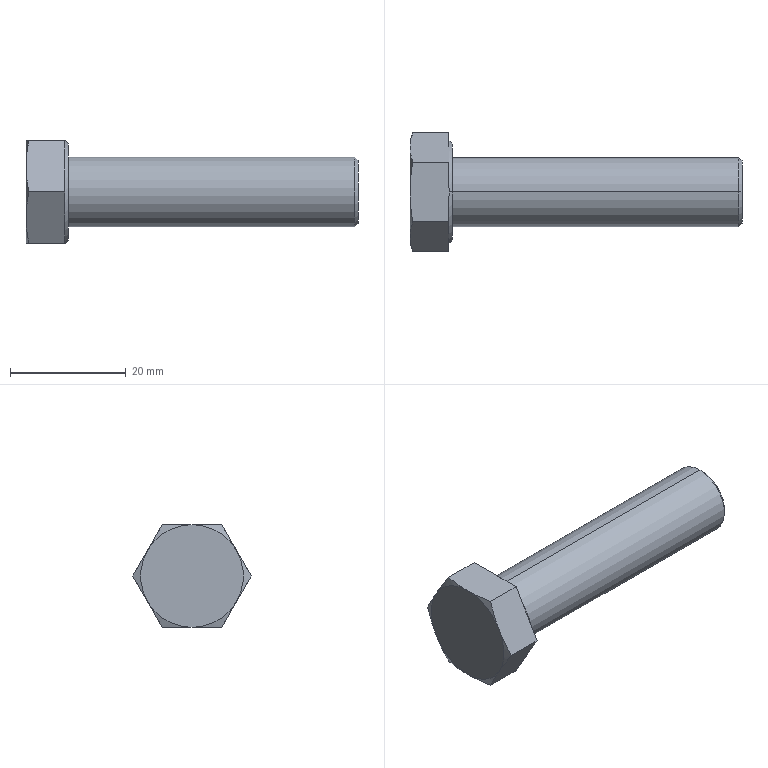Part | SolidWorks | features RevCut 3, Boss 1, Chamfer 1, Extrusion 1, Fillet 1, LPattern 1 | 1 solid | 27 faces | box 57.32 x 20.473 x 17.73 mm | volume 7614 mm3 | plane 15 | cone 10 | cylinder 2 | commonest cylinder face diameters 12 x2
STEP:
#1=CARTESIAN_POINT('',(57.32,0.,-5.4));
#2=VERTEX_POINT('',#1);
#3=CARTESIAN_POINT('',(57.32,0.,5.4));
#4=VERTEX_POINT('',#3);
#5=CARTESIAN_POINT('',(57.32,0.,0.));
#6=DIRECTION('',(1.,0.,0.));
#7=DIRECTION('',(0.,0.,-1.));
#8=AXIS2_PLACEMENT_3D('',#5,#6,#7);
#9=CIRCLE('',#8,5.4);
#10=EDGE_CURVE('',#2,#4,#9,.T.);
#11=ORIENTED_EDGE('',*,*,#10,.F.);
#12=CARTESIAN_POINT('',(56.72,0.,-6.));
#13=VERTEX_POINT('',#12);
#14=CARTESIAN_POINT('',(57.32,0.,-5.4));
#15=DIRECTION('',(-0.7071,0.,-0.7071));
#16=VECTOR('',#15,1000.);
#17=LINE('',#14,#16);
#18=EDGE_CURVE('',#2,#13,#17,.T.);
#19=ORIENTED_EDGE('',*,*,#18,.T.);
#20=CARTESIAN_POINT('',(56.72,0.,6.));
#21=VERTEX_POINT('',#20);
#22=CARTESIAN_POINT('',(56.72,0.,0.));
#23=DIRECTION('',(-1.,0.,0.));
#24=DIRECTION('',(0.,0.,-1.));
#25=AXIS2_PLACEMENT_3D('',#22,#23,#24);
#26=CIRCLE('',#25,6.);
#27=EDGE_CURVE('',#21,#13,#26,.T.);
#28=ORIENTED_EDGE('',*,*,#27,.F.);
#29=CARTESIAN_POINT('',(57.32,0.,5.4));
#30=DIRECTION('',(-0.7071,0.,0.7071));
#31=VECTOR('',#30,1000.);
#32=LINE('',#29,#31);
#33=EDGE_CURVE('',#4,#21,#32,.T.);
#34=ORIENTED_EDGE('',*,*,#33,.F.);
#35=EDGE_LOOP('',(#11,#19,#28,#34));
#36=FACE_OUTER_BOUND('',#35,.T.);
#37=CARTESIAN_POINT('',(57.32,0.,0.));
#38=DIRECTION('',(-1.,0.,0.));
#39=DIRECTION('',(0.,0.,1.));
#40=AXIS2_PLACEMENT_3D('',#37,#38,#39);
#41=CONICAL_SURFACE('',#40,5.4,0.7854);
#42=ADVANCED_FACE('',(#36),#41,.T.);
#43=ORIENTED_EDGE('',*,*,#27,.T.);
#44=CARTESIAN_POINT('',(7.32,0.,-6.));
#45=VERTEX_POINT('',#44);
#46=CARTESIAN_POINT('',(57.32,0.,-6.));
#47=DIRECTION('',(-1.,0.,0.));
#48=VECTOR('',#47,1000.);
#49=LINE('',#46,#48);
#50=EDGE_CURVE('',#13,#45,#49,.T.);
#51=ORIENTED_EDGE('',*,*,#50,.T.);
#52=CARTESIAN_POINT('',(7.32,0.,6.));
#53=VERTEX_POINT('',#52);
#54=CARTESIAN_POINT('',(7.32,0.,0.));
#55=DIRECTION('',(1.,0.,0.));
#56=DIRECTION('',(0.,0.,-1.));
#57=AXIS2_PLACEMENT_3D('',#54,#55,#56);
#58=CIRCLE('',#57,6.);
#59=EDGE_CURVE('',#45,#53,#58,.T.);
#60=ORIENTED_EDGE('',*,*,#59,.T.);
#61=CARTESIAN_POINT('',(57.32,0.,6.));
#62=DIRECTION('',(-1.,0.,0.));
#63=VECTOR('',#62,1000.);
#64=LINE('',#61,#63);
#65=EDGE_CURVE('',#21,#53,#64,.T.);
#66=ORIENTED_EDGE('',*,*,#65,.F.);
#67=EDGE_LOOP('',(#43,#51,#60,#66));
#68=FACE_OUTER_BOUND('',#67,.T.);
#69=CARTESIAN_POINT('',(57.32,0.,0.));
#70=DIRECTION('',(-1.,0.,0.));
#71=DIRECTION('',(0.,0.,1.));
#72=AXIS2_PLACEMENT_3D('',#69,#70,#71);
#73=CYLINDRICAL_SURFACE('',#72,6.);
#74=ADVANCED_FACE('',(#68),#73,.T.);
#75=CARTESIAN_POINT('',(7.32,0.,8.315));
#76=VERTEX_POINT('',#75);
#77=CARTESIAN_POINT('',(7.32,0.,-8.315));
#78=VERTEX_POINT('',#77);
#79=CARTESIAN_POINT('',(7.32,0.,0.));
#80=DIRECTION('',(-1.,0.,0.));
#81=DIRECTION('',(0.,0.,1.));
#82=AXIS2_PLACEMENT_3D('',#79,#80,#81);
#83=CIRCLE('',#82,8.315);
#84=EDGE_CURVE('',#76,#78,#83,.T.);
#85=ORIENTED_EDGE('',*,*,#84,.T.);
#86=CARTESIAN_POINT('',(6.77,0.,-8.865));
#87=VERTEX_POINT('',#86);
#88=CARTESIAN_POINT('',(6.72,0.,-8.915));
#89=DIRECTION('',(-0.7071,0.,-0.7071));
#90=VECTOR('',#89,1000.);
#91=LINE('',#88,#90);
#92=EDGE_CURVE('',#78,#87,#91,.T.);
#93=ORIENTED_EDGE('',*,*,#92,.T.);
#94=CARTESIAN_POINT('',(6.72,0.9429,-8.865));
#95=VERTEX_POINT('',#94);
#96=CARTESIAN_POINT('',(6.77,0.,-8.865));
#97=CARTESIAN_POINT('',(6.77,0.3145,-8.865));
#98=CARTESIAN_POINT('',(6.753,0.6288,-8.865));
#99=CARTESIAN_POINT('',(6.72,0.9429,-8.865));
#100=B_SPLINE_CURVE_WITH_KNOTS('',3,(#96,#97,#98,#99),.UNSPECIFIED.,.F.,.F.,(4,4),(0.004972,0.005912),.UNSPECIFIED.);
#101=EDGE_CURVE('',#87,#95,#100,.T.);
#102=ORIENTED_EDGE('',*,*,#101,.T.);
#103=CARTESIAN_POINT('',(6.72,7.206,-5.249));
#104=VERTEX_POINT('',#103);
#105=CARTESIAN_POINT('',(6.72,0.,0.));
#106=DIRECTION('',(-1.,0.,0.));
#107=DIRECTION('',(0.,0.,1.));
#108=AXIS2_PLACEMENT_3D('',#105,#106,#107);
#109=CIRCLE('',#108,8.915);
#110=EDGE_CURVE('',#104,#95,#109,.T.);
#111=ORIENTED_EDGE('',*,*,#110,.F.);
#112=CARTESIAN_POINT('',(6.72,8.149,-3.616));
#113=VERTEX_POINT('',#112);
#114=CARTESIAN_POINT('',(6.72,7.206,-5.249));
#115=CARTESIAN_POINT('',(6.786,7.52,-4.705));
#116=CARTESIAN_POINT('',(6.786,7.834,-4.16));
#117=CARTESIAN_POINT('',(6.72,8.149,-3.616));
#118=B_SPLINE_CURVE_WITH_KNOTS('',3,(#114,#115,#116,#117),.UNSPECIFIED.,.F.,.F.,(4,4),(0.000001889,0.001888),.UNSPECIFIED.);
#119=EDGE_CURVE('',#104,#113,#118,.T.);
#120=ORIENTED_EDGE('',*,*,#119,.T.);
#121=CARTESIAN_POINT('',(6.72,8.149,3.616));
#122=VERTEX_POINT('',#121);
#123=CARTESIAN_POINT('',(6.72,0.,0.));
#124=DIRECTION('',(-1.,0.,0.));
#125=DIRECTION('',(0.,0.,1.));
#126=AXIS2_PLACEMENT_3D('',#123,#124,#125);
#127=CIRCLE('',#126,8.915);
#128=EDGE_CURVE('',#122,#113,#127,.T.);
#129=ORIENTED_EDGE('',*,*,#128,.F.);
#130=CARTESIAN_POINT('',(6.72,7.206,5.249));
#131=VERTEX_POINT('',#130);
#132=CARTESIAN_POINT('',(6.72,8.149,3.616));
#133=CARTESIAN_POINT('',(6.786,7.834,4.16));
#134=CARTESIAN_POINT('',(6.786,7.52,4.705));
#135=CARTESIAN_POINT('',(6.72,7.206,5.249));
#136=B_SPLINE_CURVE_WITH_KNOTS('',3,(#132,#133,#134,#135),.UNSPECIFIED.,.F.,.F.,(4,4),(0.000001889,0.001888),.UNSPECIFIED.);
#137=EDGE_CURVE('',#122,#131,#136,.T.);
#138=ORIENTED_EDGE('',*,*,#137,.T.);
#139=CARTESIAN_POINT('',(6.72,0.9429,8.865));
#140=VERTEX_POINT('',#139);
#141=CARTESIAN_POINT('',(6.72,0.,0.));
#142=DIRECTION('',(-1.,0.,0.));
#143=DIRECTION('',(0.,0.,1.));
#144=AXIS2_PLACEMENT_3D('',#141,#142,#143);
#145=CIRCLE('',#144,8.915);
#146=EDGE_CURVE('',#140,#131,#145,.T.);
#147=ORIENTED_EDGE('',*,*,#146,.F.);
#148=CARTESIAN_POINT('',(6.77,0.,8.865));
#149=VERTEX_POINT('',#148);
#150=CARTESIAN_POINT('',(6.72,0.9429,8.865));
#151=CARTESIAN_POINT('',(6.753,0.6288,8.865));
#152=CARTESIAN_POINT('',(6.77,0.3145,8.865));
#153=CARTESIAN_POINT('',(6.77,0.,8.865));
#154=B_SPLINE_CURVE_WITH_KNOTS('',3,(#150,#151,#152,#153),.UNSPECIFIED.,.F.,.F.,(4,4),(0.004457,0.005396),.UNSPECIFIED.);
#155=EDGE_CURVE('',#140,#149,#154,.T.);
#156=ORIENTED_EDGE('',*,*,#155,.T.);
#157=CARTESIAN_POINT('',(6.72,0.,8.915));
#158=DIRECTION('',(-0.7071,0.,0.7071));
#159=VECTOR('',#158,1000.);
#160=LINE('',#157,#159);
#161=EDGE_CURVE('',#76,#149,#160,.T.);
#162=ORIENTED_EDGE('',*,*,#161,.F.);
#163=EDGE_LOOP('',(#85,#93,#102,#111,#120,#129,#138,#147,#156,#162));
#164=FACE_OUTER_BOUND('',#163,.T.);
#165=CARTESIAN_POINT('',(6.72,0.,0.));
#166=DIRECTION('',(-1.,0.,0.));
#167=DIRECTION('',(0.,0.,1.));
#168=AXIS2_PLACEMENT_3D('',#165,#166,#167);
#169=CONICAL_SURFACE('',#168,8.915,0.7854);
#170=ADVANCED_FACE('',(#164),#169,.T.);
#171=ORIENTED_EDGE('',*,*,#84,.F.);
#172=CARTESIAN_POINT('',(7.32,0.,0.));
#173=DIRECTION('',(-1.,0.,0.));
#174=DIRECTION('',(0.,0.,1.));
#175=AXIS2_PLACEMENT_3D('',#172,#173,#174);
#176=CIRCLE('',#175,8.315);
#177=EDGE_CURVE('',#78,#76,#176,.T.);
#178=ORIENTED_EDGE('',*,*,#177,.F.);
#179=EDGE_LOOP('',(#171,#178));
#180=FACE_OUTER_BOUND('',#179,.T.);
#181=CARTESIAN_POINT('',(7.32,0.,0.));
#182=DIRECTION('',(1.,0.,0.));
#183=DIRECTION('',(0.,0.,-1.));
#184=AXIS2_PLACEMENT_3D('',#181,#182,#183);
#185=CIRCLE('',#184,6.);
#186=EDGE_CURVE('',#53,#45,#185,.T.);
#187=ORIENTED_EDGE('',*,*,#186,.F.);
#188=ORIENTED_EDGE('',*,*,#59,.F.);
#189=EDGE_LOOP('',(#187,#188));
#190=FACE_BOUND('',#189,.T.);
#191=CARTESIAN_POINT('',(7.32,-15.355,-8.865));
#192=DIRECTION('',(1.,0.,0.));
#193=DIRECTION('',(0.,0.,-1.));
#194=AXIS2_PLACEMENT_3D('',#191,#192,#193);
#195=PLANE('',#194);
#196=ADVANCED_FACE('',(#180,#190),#195,.T.);
#197=CARTESIAN_POINT('',(0.4992,-10.236,0.));
#198=VERTEX_POINT('',#197);
#199=CARTESIAN_POINT('',(0.,-7.677,4.433));
#200=VERTEX_POINT('',#199);
#201=CARTESIAN_POINT('',(0.4992,-10.236,0.));
#202=CARTESIAN_POINT('',(0.3439,-9.81,0.7388));
#203=CARTESIAN_POINT('',(0.2179,-9.383,1.478));
#204=CARTESIAN_POINT('',(0.04564,-8.53,2.955));
#205=CARTESIAN_POINT('',(0.,-8.104,3.694));
#206=CARTESIAN_POINT('',(0.,-7.677,4.433));
#207=B_SPLINE_CURVE_WITH_KNOTS('',3,(#201,#202,#203,#204,#205,#206),.UNSPECIFIED.,.F.,.F.,(4,2,4),(0.000000231,0.002559,0.005118),.UNSPECIFIED.);
#208=EDGE_CURVE('',#198,#200,#207,.T.);
#209=ORIENTED_EDGE('',*,*,#208,.F.);
#210=CARTESIAN_POINT('',(6.72,-10.236,0.));
#211=VERTEX_POINT('',#210);
#212=CARTESIAN_POINT('',(7.32,-10.236,0.));
#213=DIRECTION('',(-1.,0.,0.));
#214=VECTOR('',#213,1000.);
#215=LINE('',#212,#214);
#216=EDGE_CURVE('',#211,#198,#215,.T.);
#217=ORIENTED_EDGE('',*,*,#216,.F.);
#218=CARTESIAN_POINT('',(6.72,-8.149,3.616));
#219=VERTEX_POINT('',#218);
#220=CARTESIAN_POINT('',(6.72,-5.118,8.865));
#221=DIRECTION('',(0.,-0.5,-0.866));
#222=VECTOR('',#221,1000.);
#223=LINE('',#220,#222);
#224=EDGE_CURVE('',#219,#211,#223,.T.);
#225=ORIENTED_EDGE('',*,*,#224,.F.);
#226=CARTESIAN_POINT('',(6.72,-7.206,5.249));
#227=VERTEX_POINT('',#226);
#228=CARTESIAN_POINT('',(6.72,-7.206,5.249));
#229=CARTESIAN_POINT('',(6.786,-7.52,4.705));
#230=CARTESIAN_POINT('',(6.786,-7.834,4.16));
#231=CARTESIAN_POINT('',(6.72,-8.149,3.616));
#232=B_SPLINE_CURVE_WITH_KNOTS('',3,(#228,#229,#230,#231),.UNSPECIFIED.,.F.,.F.,(4,4),(0.000001889,0.001888),.UNSPECIFIED.);
#233=EDGE_CURVE('',#227,#219,#232,.T.);
#234=ORIENTED_EDGE('',*,*,#233,.F.);
#235=CARTESIAN_POINT('',(6.72,-5.118,8.865));
#236=VERTEX_POINT('',#235);
#237=CARTESIAN_POINT('',(6.72,-5.118,8.865));
#238=DIRECTION('',(0.,-0.5,-0.866));
#239=VECTOR('',#238,1000.);
#240=LINE('',#237,#239);
#241=EDGE_CURVE('',#236,#227,#240,.T.);
#242=ORIENTED_EDGE('',*,*,#241,.F.);
#243=CARTESIAN_POINT('',(0.4992,-5.118,8.865));
#244=VERTEX_POINT('',#243);
#245=CARTESIAN_POINT('',(7.32,-5.118,8.865));
#246=DIRECTION('',(-1.,0.,0.));
#247=VECTOR('',#246,1000.);
#248=LINE('',#245,#247);
#249=EDGE_CURVE('',#236,#244,#248,.T.);
#250=ORIENTED_EDGE('',*,*,#249,.T.);
#251=CARTESIAN_POINT('',(0.,-7.677,4.433));
#252=CARTESIAN_POINT('',(0.,-7.251,5.171));
#253=CARTESIAN_POINT('',(0.04564,-6.824,5.91));
#254=CARTESIAN_POINT('',(0.2179,-5.971,7.387));
#255=CARTESIAN_POINT('',(0.3439,-5.545,8.126));
#256=CARTESIAN_POINT('',(0.4992,-5.118,8.865));
#257=B_SPLINE_CURVE_WITH_KNOTS('',3,(#251,#252,#253,#254,#255,#256),.UNSPECIFIED.,.F.,.F.,(4,2,4),(0.005118,0.007678,0.01024),.UNSPECIFIED.);
#258=EDGE_CURVE('',#200,#244,#257,.T.);
#259=ORIENTED_EDGE('',*,*,#258,.F.);
#260=EDGE_LOOP('',(#209,#217,#225,#234,#242,#250,#259));
#261=FACE_OUTER_BOUND('',#260,.T.);
#262=CARTESIAN_POINT('',(7.32,-5.118,8.865));
#263=DIRECTION('',(0.,0.866,-0.5));
#264=DIRECTION('',(0.,0.5,0.866));
#265=AXIS2_PLACEMENT_3D('',#262,#263,#264);
#266=PLANE('',#265);
#267=ADVANCED_FACE('',(#261),#266,.F.);
#268=CARTESIAN_POINT('',(0.4992,-5.118,-8.865));
#269=VERTEX_POINT('',#268);
#270=CARTESIAN_POINT('',(0.,-7.677,-4.432));
#271=VERTEX_POINT('',#270);
#272=CARTESIAN_POINT('',(0.4992,-5.118,-8.865));
#273=CARTESIAN_POINT('',(0.3439,-5.545,-8.126));
#274=CARTESIAN_POINT('',(0.2179,-5.971,-7.387));
#275=CARTESIAN_POINT('',(0.04564,-6.824,-5.91));
#276=CARTESIAN_POINT('',(0.,-7.251,-5.171));
#277=CARTESIAN_POINT('',(0.,-7.677,-4.432));
#278=B_SPLINE_CURVE_WITH_KNOTS('',3,(#272,#273,#274,#275,#276,#277),.UNSPECIFIED.,.F.,.F.,(4,2,4),(0.000000231,0.002559,0.005118),.UNSPECIFIED.);
#279=EDGE_CURVE('',#269,#271,#278,.T.);
#280=ORIENTED_EDGE('',*,*,#279,.F.);
#281=CARTESIAN_POINT('',(6.72,-5.118,-8.865));
#282=VERTEX_POINT('',#281);
#283=CARTESIAN_POINT('',(7.32,-5.118,-8.865));
#284=DIRECTION('',(-1.,0.,0.));
#285=VECTOR('',#284,1000.);
#286=LINE('',#283,#285);
#287=EDGE_CURVE('',#282,#269,#286,.T.);
#288=ORIENTED_EDGE('',*,*,#287,.F.);
#289=CARTESIAN_POINT('',(6.72,-7.206,-5.249));
#290=VERTEX_POINT('',#289);
#291=CARTESIAN_POINT('',(6.72,-10.236,0.));
#292=DIRECTION('',(0.,0.5,-0.866));
#293=VECTOR('',#292,1000.);
#294=LINE('',#291,#293);
#295=EDGE_CURVE('',#290,#282,#294,.T.);
#296=ORIENTED_EDGE('',*,*,#295,.F.);
#297=CARTESIAN_POINT('',(6.72,-8.149,-3.616));
#298=VERTEX_POINT('',#297);
#299=CARTESIAN_POINT('',(6.72,-8.149,-3.616));
#300=CARTESIAN_POINT('',(6.786,-7.834,-4.16));
#301=CARTESIAN_POINT('',(6.786,-7.52,-4.705));
#302=CARTESIAN_POINT('',(6.72,-7.206,-5.249));
#303=B_SPLINE_CURVE_WITH_KNOTS('',3,(#299,#300,#301,#302),.UNSPECIFIED.,.F.,.F.,(4,4),(0.000001889,0.001888),.UNSPECIFIED.);
#304=EDGE_CURVE('',#298,#290,#303,.T.);
#305=ORIENTED_EDGE('',*,*,#304,.F.);
#306=CARTESIAN_POINT('',(6.72,-10.236,0.));
#307=DIRECTION('',(0.,0.5,-0.866));
#308=VECTOR('',#307,1000.);
#309=LINE('',#306,#308);
#310=EDGE_CURVE('',#211,#298,#309,.T.);
#311=ORIENTED_EDGE('',*,*,#310,.F.);
#312=ORIENTED_EDGE('',*,*,#216,.T.);
#313=CARTESIAN_POINT('',(0.,-7.677,-4.432));
#314=CARTESIAN_POINT('',(0.,-8.104,-3.694));
#315=CARTESIAN_POINT('',(0.04564,-8.53,-2.955));
#316=CARTESIAN_POINT('',(0.2179,-9.383,-1.477));
#317=CARTESIAN_POINT('',(0.3439,-9.81,-0.7387));
#318=CARTESIAN_POINT('',(0.4992,-10.236,0.));
#319=B_SPLINE_CURVE_WITH_KNOTS('',3,(#313,#314,#315,#316,#317,#318),.UNSPECIFIED.,.F.,.F.,(4,2,4),(0.005118,0.007678,0.01024),.UNSPECIFIED.);
#320=EDGE_CURVE('',#271,#198,#319,.T.);
#321=ORIENTED_EDGE('',*,*,#320,.F.);
#322=EDGE_LOOP('',(#280,#288,#296,#305,#311,#312,#321));
#323=FACE_OUTER_BOUND('',#322,.T.);
#324=CARTESIAN_POINT('',(7.32,-10.236,0.));
#325=DIRECTION('',(0.,0.866,0.5));
#326=DIRECTION('',(0.,-0.5,0.866));
#327=AXIS2_PLACEMENT_3D('',#324,#325,#326);
#328=PLANE('',#327);
#329=ADVANCED_FACE('',(#323),#328,.F.);
#330=CARTESIAN_POINT('',(0.4992,5.118,-8.865));
#331=VERTEX_POINT('',#330);
#332=CARTESIAN_POINT('',(0.,0.,-8.865));
#333=VERTEX_POINT('',#332);
#334=CARTESIAN_POINT('',(0.4992,5.118,-8.865));
#335=CARTESIAN_POINT('',(0.3443,4.267,-8.865));
#336=CARTESIAN_POINT('',(0.2182,3.415,-8.865));
#337=CARTESIAN_POINT('',(0.04582,1.709,-8.865));
#338=CARTESIAN_POINT('',(0.,0.8548,-8.865));
#339=CARTESIAN_POINT('',(0.,0.,-8.865));
#340=B_SPLINE_CURVE_WITH_KNOTS('',3,(#334,#335,#336,#337,#338,#339),.UNSPECIFIED.,.F.,.F.,(4,2,4),(0.01846,0.02104,0.02362),.UNSPECIFIED.);
#341=EDGE_CURVE('',#331,#333,#340,.T.);
#342=ORIENTED_EDGE('',*,*,#341,.F.);
#343=CARTESIAN_POINT('',(6.72,5.118,-8.865));
#344=VERTEX_POINT('',#343);
#345=CARTESIAN_POINT('',(7.32,5.118,-8.865));
#346=DIRECTION('',(-1.,0.,0.));
#347=VECTOR('',#346,1000.);
#348=LINE('',#345,#347);
#349=EDGE_CURVE('',#344,#331,#348,.T.);
#350=ORIENTED_EDGE('',*,*,#349,.F.);
#351=CARTESIAN_POINT('',(6.72,-5.118,-8.865));
#352=DIRECTION('',(0.,1.,0.));
#353=VECTOR('',#352,1000.);
#354=LINE('',#351,#353);
#355=EDGE_CURVE('',#95,#344,#354,.T.);
#356=ORIENTED_EDGE('',*,*,#355,.F.);
#357=ORIENTED_EDGE('',*,*,#101,.F.);
#358=CARTESIAN_POINT('',(6.72,-0.9429,-8.865));
#359=VERTEX_POINT('',#358);
#360=CARTESIAN_POINT('',(6.72,-0.9429,-8.865));
#361=CARTESIAN_POINT('',(6.753,-0.6284,-8.865));
#362=CARTESIAN_POINT('',(6.77,-0.3141,-8.865));
#363=CARTESIAN_POINT('',(6.77,0.,-8.865));
#364=B_SPLINE_CURVE_WITH_KNOTS('',3,(#360,#361,#362,#363),.UNSPECIFIED.,.F.,.F.,(4,4),(0.004033,0.004972),.UNSPECIFIED.);
#365=EDGE_CURVE('',#359,#87,#364,.T.);
#366=ORIENTED_EDGE('',*,*,#365,.F.);
#367=CARTESIAN_POINT('',(6.72,-5.118,-8.865));
#368=DIRECTION('',(0.,1.,0.));
#369=VECTOR('',#368,1000.);
#370=LINE('',#367,#369);
#371=EDGE_CURVE('',#282,#359,#370,.T.);
#372=ORIENTED_EDGE('',*,*,#371,.F.);
#373=ORIENTED_EDGE('',*,*,#287,.T.);
#374=CARTESIAN_POINT('',(0.,0.,-8.865));
#375=CARTESIAN_POINT('',(0.,-0.8523,-8.865));
#376=CARTESIAN_POINT('',(0.04558,-1.706,-8.865));
#377=CARTESIAN_POINT('',(0.2181,-3.414,-8.865));
#378=CARTESIAN_POINT('',(0.3449,-4.271,-8.865));
#379=CARTESIAN_POINT('',(0.4992,-5.118,-8.865));
#380=B_SPLINE_CURVE_WITH_KNOTS('',3,(#374,#375,#376,#377,#378,#379),.UNSPECIFIED.,.F.,.F.,(4,2,4),(0.02362,0.02619,0.02876),.UNSPECIFIED.);
#381=EDGE_CURVE('',#333,#269,#380,.T.);
#382=ORIENTED_EDGE('',*,*,#381,.F.);
#383=EDGE_LOOP('',(#342,#350,#356,#357,#366,#372,#373,#382));
#384=FACE_OUTER_BOUND('',#383,.T.);
#385=CARTESIAN_POINT('',(7.32,-5.118,-8.865));
#386=DIRECTION('',(0.,0.,1.));
#387=DIRECTION('',(0.,-1.,0.));
#388=AXIS2_PLACEMENT_3D('',#385,#386,#387);
#389=PLANE('',#388);
#390=ADVANCED_FACE('',(#384),#389,.F.);
#391=CARTESIAN_POINT('',(0.4992,10.236,0.));
#392=VERTEX_POINT('',#391);
#393=CARTESIAN_POINT('',(0.,7.677,-4.432));
#394=VERTEX_POINT('',#393);
#395=CARTESIAN_POINT('',(0.4992,10.236,0.));
#396=CARTESIAN_POINT('',(0.3439,9.81,-0.7388));
#397=CARTESIAN_POINT('',(0.2179,9.383,-1.478));
#398=CARTESIAN_POINT('',(0.04564,8.53,-2.955));
#399=CARTESIAN_POINT('',(0.,8.104,-3.694));
#400=CARTESIAN_POINT('',(0.,7.677,-4.432));
#401=B_SPLINE_CURVE_WITH_KNOTS('',3,(#395,#396,#397,#398,#399,#400),.UNSPECIFIED.,.F.,.F.,(4,2,4),(0.000000231,0.002559,0.005118),.UNSPECIFIED.);
#402=EDGE_CURVE('',#392,#394,#401,.T.);
#403=ORIENTED_EDGE('',*,*,#402,.F.);
#404=CARTESIAN_POINT('',(6.72,10.236,0.));
#405=VERTEX_POINT('',#404);
#406=CARTESIAN_POINT('',(7.32,10.236,0.));
#407=DIRECTION('',(-1.,0.,0.));
#408=VECTOR('',#407,1000.);
#409=LINE('',#406,#408);
#410=EDGE_CURVE('',#405,#392,#409,.T.);
#411=ORIENTED_EDGE('',*,*,#410,.F.);
#412=CARTESIAN_POINT('',(6.72,5.118,-8.865));
#413=DIRECTION('',(0.,0.5,0.866));
#414=VECTOR('',#413,1000.);
#415=LINE('',#412,#414);
#416=EDGE_CURVE('',#113,#405,#415,.T.);
#417=ORIENTED_EDGE('',*,*,#416,.F.);
#418=ORIENTED_EDGE('',*,*,#119,.F.);
#419=CARTESIAN_POINT('',(6.72,5.118,-8.865));
#420=DIRECTION('',(0.,0.5,0.866));
#421=VECTOR('',#420,1000.);
#422=LINE('',#419,#421);
#423=EDGE_CURVE('',#344,#104,#422,.T.);
#424=ORIENTED_EDGE('',*,*,#423,.F.);
#425=ORIENTED_EDGE('',*,*,#349,.T.);
#426=CARTESIAN_POINT('',(0.,7.677,-4.432));
#427=CARTESIAN_POINT('',(0.,7.251,-5.171));
#428=CARTESIAN_POINT('',(0.04564,6.824,-5.91));
#429=CARTESIAN_POINT('',(0.2179,5.971,-7.387));
#430=CARTESIAN_POINT('',(0.3439,5.545,-8.126));
#431=CARTESIAN_POINT('',(0.4992,5.118,-8.865));
#432=B_SPLINE_CURVE_WITH_KNOTS('',3,(#426,#427,#428,#429,#430,#431),.UNSPECIFIED.,.F.,.F.,(4,2,4),(0.005118,0.007678,0.01024),.UNSPECIFIED.);
#433=EDGE_CURVE('',#394,#331,#432,.T.);
#434=ORIENTED_EDGE('',*,*,#433,.F.);
#435=EDGE_LOOP('',(#403,#411,#417,#418,#424,#425,#434));
#436=FACE_OUTER_BOUND('',#435,.T.);
#437=CARTESIAN_POINT('',(7.32,5.118,-8.865));
#438=DIRECTION('',(0.,-0.866,0.5));
#439=DIRECTION('',(0.,-0.5,-0.866));
#440=AXIS2_PLACEMENT_3D('',#437,#438,#439);
#441=PLANE('',#440);
#442=ADVANCED_FACE('',(#436),#441,.F.);
#443=CARTESIAN_POINT('',(0.4992,5.118,8.865));
#444=VERTEX_POINT('',#443);
#445=CARTESIAN_POINT('',(0.,7.677,4.432));
#446=VERTEX_POINT('',#445);
#447=CARTESIAN_POINT('',(0.4992,5.118,8.865));
#448=CARTESIAN_POINT('',(0.3439,5.545,8.126));
#449=CARTESIAN_POINT('',(0.2179,5.971,7.388));
#450=CARTESIAN_POINT('',(0.04564,6.824,5.91));
#451=CARTESIAN_POINT('',(0.,7.251,5.171));
#452=CARTESIAN_POINT('',(0.,7.677,4.432));
#453=B_SPLINE_CURVE_WITH_KNOTS('',3,(#447,#448,#449,#450,#451,#452),.UNSPECIFIED.,.F.,.F.,(4,2,4),(0.000000231,0.002559,0.005118),.UNSPECIFIED.);
#454=EDGE_CURVE('',#444,#446,#453,.T.);
#455=ORIENTED_EDGE('',*,*,#454,.F.);
#456=CARTESIAN_POINT('',(6.72,5.118,8.865));
#457=VERTEX_POINT('',#456);
#458=CARTESIAN_POINT('',(7.32,5.118,8.865));
#459=DIRECTION('',(-1.,0.,0.));
#460=VECTOR('',#459,1000.);
#461=LINE('',#458,#460);
#462=EDGE_CURVE('',#457,#444,#461,.T.);
#463=ORIENTED_EDGE('',*,*,#462,.F.);
#464=CARTESIAN_POINT('',(6.72,10.236,0.));
#465=DIRECTION('',(0.,-0.5,0.866));
#466=VECTOR('',#465,1000.);
#467=LINE('',#464,#466);
#468=EDGE_CURVE('',#131,#457,#467,.T.);
#469=ORIENTED_EDGE('',*,*,#468,.F.);
#470=ORIENTED_EDGE('',*,*,#137,.F.);
#471=CARTESIAN_POINT('',(6.72,10.236,0.));
#472=DIRECTION('',(0.,-0.5,0.866));
#473=VECTOR('',#472,1000.);
#474=LINE('',#471,#473);
#475=EDGE_CURVE('',#405,#122,#474,.T.);
#476=ORIENTED_EDGE('',*,*,#475,.F.);
#477=ORIENTED_EDGE('',*,*,#410,.T.);
#478=CARTESIAN_POINT('',(0.,7.677,4.432));
#479=CARTESIAN_POINT('',(0.,8.104,3.694));
#480=CARTESIAN_POINT('',(0.04564,8.53,2.955));
#481=CARTESIAN_POINT('',(0.2179,9.383,1.477));
#482=CARTESIAN_POINT('',(0.3439,9.81,0.7387));
#483=CARTESIAN_POINT('',(0.4992,10.236,0.));
#484=B_SPLINE_CURVE_WITH_KNOTS('',3,(#478,#479,#480,#481,#482,#483),.UNSPECIFIED.,.F.,.F.,(4,2,4),(0.005118,0.007678,0.01024),.UNSPECIFIED.);
#485=EDGE_CURVE('',#446,#392,#484,.T.);
#486=ORIENTED_EDGE('',*,*,#485,.F.);
#487=EDGE_LOOP('',(#455,#463,#469,#470,#476,#477,#486));
#488=FACE_OUTER_BOUND('',#487,.T.);
#489=CARTESIAN_POINT('',(7.32,10.236,0.));
#490=DIRECTION('',(0.,-0.866,-0.5));
#491=DIRECTION('',(0.,0.5,-0.866));
#492=AXIS2_PLACEMENT_3D('',#489,#490,#491);
#493=PLANE('',#492);
#494=ADVANCED_FACE('',(#488),#493,.F.);
#495=CARTESIAN_POINT('',(0.,0.,8.865));
#496=VERTEX_POINT('',#495);
#497=CARTESIAN_POINT('',(0.4992,-5.118,8.865));
#498=CARTESIAN_POINT('',(0.3449,-4.271,8.865));
#499=CARTESIAN_POINT('',(0.2181,-3.414,8.865));
#500=CARTESIAN_POINT('',(0.04558,-1.706,8.865));
#501=CARTESIAN_POINT('',(0.,-0.8523,8.865));
#502=CARTESIAN_POINT('',(0.,0.,8.865));
#503=B_SPLINE_CURVE_WITH_KNOTS('',3,(#497,#498,#499,#500,#501,#502),.UNSPECIFIED.,.F.,.F.,(4,2,4),(0.008707,0.01129,0.01387),.UNSPECIFIED.);
#504=EDGE_CURVE('',#244,#496,#503,.T.);
#505=ORIENTED_EDGE('',*,*,#504,.F.);
#506=ORIENTED_EDGE('',*,*,#249,.F.);
#507=CARTESIAN_POINT('',(6.72,-0.9429,8.865));
#508=VERTEX_POINT('',#507);
#509=CARTESIAN_POINT('',(6.72,5.118,8.865));
#510=DIRECTION('',(0.,-1.,0.));
#511=VECTOR('',#510,1000.);
#512=LINE('',#509,#511);
#513=EDGE_CURVE('',#508,#236,#512,.T.);
#514=ORIENTED_EDGE('',*,*,#513,.F.);
#515=CARTESIAN_POINT('',(6.77,0.,8.865));
#516=CARTESIAN_POINT('',(6.77,-0.3141,8.865));
#517=CARTESIAN_POINT('',(6.753,-0.6284,8.865));
#518=CARTESIAN_POINT('',(6.72,-0.9429,8.865));
#519=B_SPLINE_CURVE_WITH_KNOTS('',3,(#515,#516,#517,#518),.UNSPECIFIED.,.F.,.F.,(4,4),(0.005396,0.006334),.UNSPECIFIED.);
#520=EDGE_CURVE('',#149,#508,#519,.T.);
#521=ORIENTED_EDGE('',*,*,#520,.F.);
#522=ORIENTED_EDGE('',*,*,#155,.F.);
#523=CARTESIAN_POINT('',(6.72,5.118,8.865));
#524=DIRECTION('',(0.,-1.,0.));
#525=VECTOR('',#524,1000.);
#526=LINE('',#523,#525);
#527=EDGE_CURVE('',#457,#140,#526,.T.);
#528=ORIENTED_EDGE('',*,*,#527,.F.);
#529=ORIENTED_EDGE('',*,*,#462,.T.);
#530=CARTESIAN_POINT('',(0.,0.,8.865));
#531=CARTESIAN_POINT('',(0.,0.8548,8.865));
#532=CARTESIAN_POINT('',(0.04582,1.709,8.865));
#533=CARTESIAN_POINT('',(0.2182,3.415,8.865));
#534=CARTESIAN_POINT('',(0.3443,4.267,8.865));
#535=CARTESIAN_POINT('',(0.4992,5.118,8.865));
#536=B_SPLINE_CURVE_WITH_KNOTS('',3,(#530,#531,#532,#533,#534,#535),.UNSPECIFIED.,.F.,.F.,(4,2,4),(0.01387,0.01645,0.01904),.UNSPECIFIED.);
#537=EDGE_CURVE('',#496,#444,#536,.T.);
#538=ORIENTED_EDGE('',*,*,#537,.F.);
#539=EDGE_LOOP('',(#505,#506,#514,#521,#522,#528,#529,#538));
#540=FACE_OUTER_BOUND('',#539,.T.);
#541=CARTESIAN_POINT('',(7.32,5.118,8.865));
#542=DIRECTION('',(0.,0.,-1.));
#543=DIRECTION('',(-1.,0.,0.));
#544=AXIS2_PLACEMENT_3D('',#541,#542,#543);
#545=PLANE('',#544);
#546=ADVANCED_FACE('',(#540),#545,.F.);
#547=ORIENTED_EDGE('',*,*,#224,.T.);
#548=ORIENTED_EDGE('',*,*,#310,.T.);
#549=CARTESIAN_POINT('',(6.72,0.,0.));
#550=DIRECTION('',(-1.,0.,0.));
#551=DIRECTION('',(0.,0.,1.));
#552=AXIS2_PLACEMENT_3D('',#549,#550,#551);
#553=CIRCLE('',#552,8.915);
#554=EDGE_CURVE('',#298,#219,#553,.T.);
#555=ORIENTED_EDGE('',*,*,#554,.T.);
#556=EDGE_LOOP('',(#547,#548,#555));
#557=FACE_OUTER_BOUND('',#556,.T.);
#558=CARTESIAN_POINT('',(6.72,8.915,0.));
#559=DIRECTION('',(1.,0.,0.));
#560=DIRECTION('',(0.,0.,-1.));
#561=AXIS2_PLACEMENT_3D('',#558,#559,#560);
#562=PLANE('',#561);
#563=ADVANCED_FACE('',(#557),#562,.T.);
#564=ORIENTED_EDGE('',*,*,#295,.T.);
#565=ORIENTED_EDGE('',*,*,#371,.T.);
#566=CARTESIAN_POINT('',(6.72,0.,0.));
#567=DIRECTION('',(-1.,0.,0.));
#568=DIRECTION('',(0.,0.,1.));
#569=AXIS2_PLACEMENT_3D('',#566,#567,#568);
#570=CIRCLE('',#569,8.915);
#571=EDGE_CURVE('',#359,#290,#570,.T.);
#572=ORIENTED_EDGE('',*,*,#571,.T.);
#573=EDGE_LOOP('',(#564,#565,#572));
#574=FACE_OUTER_BOUND('',#573,.T.);
#575=CARTESIAN_POINT('',(6.72,8.915,0.));
#576=DIRECTION('',(1.,0.,0.));
#577=DIRECTION('',(0.,0.,-1.));
#578=AXIS2_PLACEMENT_3D('',#575,#576,#577);
#579=PLANE('',#578);
#580=ADVANCED_FACE('',(#574),#579,.T.);
#581=ORIENTED_EDGE('',*,*,#355,.T.);
#582=ORIENTED_EDGE('',*,*,#423,.T.);
#583=ORIENTED_EDGE('',*,*,#110,.T.);
#584=EDGE_LOOP('',(#581,#582,#583));
#585=FACE_OUTER_BOUND('',#584,.T.);
#586=CARTESIAN_POINT('',(6.72,8.915,0.));
#587=DIRECTION('',(1.,0.,0.));
#588=DIRECTION('',(0.,0.,-1.));
#589=AXIS2_PLACEMENT_3D('',#586,#587,#588);
#590=PLANE('',#589);
#591=ADVANCED_FACE('',(#585),#590,.T.);
#592=ORIENTED_EDGE('',*,*,#416,.T.);
#593=ORIENTED_EDGE('',*,*,#475,.T.);
#594=ORIENTED_EDGE('',*,*,#128,.T.);
#595=EDGE_LOOP('',(#592,#593,#594));
#596=FACE_OUTER_BOUND('',#595,.T.);
#597=CARTESIAN_POINT('',(6.72,8.915,0.));
#598=DIRECTION('',(1.,0.,0.));
#599=DIRECTION('',(0.,0.,-1.));
#600=AXIS2_PLACEMENT_3D('',#597,#598,#599);
#601=PLANE('',#600);
#602=ADVANCED_FACE('',(#596),#601,.T.);
#603=ORIENTED_EDGE('',*,*,#468,.T.);
#604=ORIENTED_EDGE('',*,*,#527,.T.);
#605=ORIENTED_EDGE('',*,*,#146,.T.);
#606=EDGE_LOOP('',(#603,#604,#605));
#607=FACE_OUTER_BOUND('',#606,.T.);
#608=CARTESIAN_POINT('',(6.72,8.915,0.));
#609=DIRECTION('',(1.,0.,0.));
#610=DIRECTION('',(0.,0.,-1.));
#611=AXIS2_PLACEMENT_3D('',#608,#609,#610);
#612=PLANE('',#611);
#613=ADVANCED_FACE('',(#607),#612,.T.);
#614=ORIENTED_EDGE('',*,*,#241,.T.);
#615=CARTESIAN_POINT('',(6.72,0.,0.));
#616=DIRECTION('',(-1.,0.,0.));
#617=DIRECTION('',(0.,0.,1.));
#618=AXIS2_PLACEMENT_3D('',#615,#616,#617);
#619=CIRCLE('',#618,8.915);
#620=EDGE_CURVE('',#227,#508,#619,.T.);
#621=ORIENTED_EDGE('',*,*,#620,.T.);
#622=ORIENTED_EDGE('',*,*,#513,.T.);
#623=EDGE_LOOP('',(#614,#621,#622));
#624=FACE_OUTER_BOUND('',#623,.T.);
#625=CARTESIAN_POINT('',(6.72,8.915,0.));
#626=DIRECTION('',(1.,0.,0.));
#627=DIRECTION('',(0.,0.,-1.));
#628=AXIS2_PLACEMENT_3D('',#625,#626,#627);
#629=PLANE('',#628);
#630=ADVANCED_FACE('',(#624),#629,.T.);
#631=ORIENTED_EDGE('',*,*,#92,.F.);
#632=ORIENTED_EDGE('',*,*,#177,.T.);
#633=ORIENTED_EDGE('',*,*,#161,.T.);
#634=ORIENTED_EDGE('',*,*,#520,.T.);
#635=ORIENTED_EDGE('',*,*,#620,.F.);
#636=ORIENTED_EDGE('',*,*,#233,.T.);
#637=ORIENTED_EDGE('',*,*,#554,.F.);
#638=ORIENTED_EDGE('',*,*,#304,.T.);
#639=ORIENTED_EDGE('',*,*,#571,.F.);
#640=ORIENTED_EDGE('',*,*,#365,.T.);
#641=EDGE_LOOP('',(#631,#632,#633,#634,#635,#636,#637,#638,#639,#640));
#642=FACE_OUTER_BOUND('',#641,.T.);
#643=CARTESIAN_POINT('',(6.72,0.,0.));
#644=DIRECTION('',(-1.,0.,0.));
#645=DIRECTION('',(0.,0.,1.));
#646=AXIS2_PLACEMENT_3D('',#643,#644,#645);
#647=CONICAL_SURFACE('',#646,8.915,0.7854);
#648=ADVANCED_FACE('',(#642),#647,.T.);
#649=ORIENTED_EDGE('',*,*,#381,.T.);
#650=ORIENTED_EDGE('',*,*,#279,.T.);
#651=CARTESIAN_POINT('',(0.,0.,0.));
#652=DIRECTION('',(1.,0.,0.));
#653=DIRECTION('',(0.,0.,-1.));
#654=AXIS2_PLACEMENT_3D('',#651,#652,#653);
#655=CIRCLE('',#654,8.865);
#656=EDGE_CURVE('',#271,#333,#655,.T.);
#657=ORIENTED_EDGE('',*,*,#656,.T.);
#658=EDGE_LOOP('',(#649,#650,#657));
#659=FACE_OUTER_BOUND('',#658,.T.);
#660=CARTESIAN_POINT('',(0.,0.,0.));
#661=DIRECTION('',(1.,0.,0.));
#662=DIRECTION('',(0.,0.,-1.));
#663=AXIS2_PLACEMENT_3D('',#660,#661,#662);
#664=CONICAL_SURFACE('',#663,8.865,1.222);
#665=ADVANCED_FACE('',(#659),#664,.T.);
#666=ORIENTED_EDGE('',*,*,#320,.T.);
#667=ORIENTED_EDGE('',*,*,#208,.T.);
#668=CARTESIAN_POINT('',(0.,0.,0.));
#669=DIRECTION('',(1.,0.,0.));
#670=DIRECTION('',(0.,0.,-1.));
#671=AXIS2_PLACEMENT_3D('',#668,#669,#670);
#672=CIRCLE('',#671,8.865);
#673=EDGE_CURVE('',#200,#271,#672,.T.);
#674=ORIENTED_EDGE('',*,*,#673,.T.);
#675=EDGE_LOOP('',(#666,#667,#674));
#676=FACE_OUTER_BOUND('',#675,.T.);
#677=CARTESIAN_POINT('',(0.,0.,0.));
#678=DIRECTION('',(1.,0.,0.));
#679=DIRECTION('',(0.,0.,-1.));
#680=AXIS2_PLACEMENT_3D('',#677,#678,#679);
#681=CONICAL_SURFACE('',#680,8.865,1.222);
#682=ADVANCED_FACE('',(#676),#681,.T.);
#683=ORIENTED_EDGE('',*,*,#258,.T.);
#684=ORIENTED_EDGE('',*,*,#504,.T.);
#685=CARTESIAN_POINT('',(0.,0.,0.));
#686=DIRECTION('',(1.,0.,0.));
#687=DIRECTION('',(0.,0.,-1.));
#688=AXIS2_PLACEMENT_3D('',#685,#686,#687);
#689=CIRCLE('',#688,8.865);
#690=EDGE_CURVE('',#496,#200,#689,.T.);
#691=ORIENTED_EDGE('',*,*,#690,.T.);
#692=EDGE_LOOP('',(#683,#684,#691));
#693=FACE_OUTER_BOUND('',#692,.T.);
#694=CARTESIAN_POINT('',(0.,0.,0.));
#695=DIRECTION('',(1.,0.,0.));
#696=DIRECTION('',(0.,0.,-1.));
#697=AXIS2_PLACEMENT_3D('',#694,#695,#696);
#698=CONICAL_SURFACE('',#697,8.865,1.222);
#699=ADVANCED_FACE('',(#693),#698,.T.);
#700=ORIENTED_EDGE('',*,*,#454,.T.);
#701=CARTESIAN_POINT('',(0.,0.,0.));
#702=DIRECTION('',(-1.,0.,0.));
#703=DIRECTION('',(0.,0.,1.));
#704=AXIS2_PLACEMENT_3D('',#701,#702,#703);
#705=CIRCLE('',#704,8.865);
#706=EDGE_CURVE('',#496,#446,#705,.T.);
#707=ORIENTED_EDGE('',*,*,#706,.F.);
#708=ORIENTED_EDGE('',*,*,#537,.T.);
#709=EDGE_LOOP('',(#700,#707,#708));
#710=FACE_OUTER_BOUND('',#709,.T.);
#711=CARTESIAN_POINT('',(0.,0.,0.));
#712=DIRECTION('',(1.,0.,0.));
#713=DIRECTION('',(0.,0.,-1.));
#714=AXIS2_PLACEMENT_3D('',#711,#712,#713);
#715=CONICAL_SURFACE('',#714,8.865,1.222);
#716=ADVANCED_FACE('',(#710),#715,.T.);
#717=ORIENTED_EDGE('',*,*,#402,.T.);
#718=CARTESIAN_POINT('',(0.,0.,0.));
#719=DIRECTION('',(1.,0.,0.));
#720=DIRECTION('',(0.,0.,-1.));
#721=AXIS2_PLACEMENT_3D('',#718,#719,#720);
#722=CIRCLE('',#721,8.865);
#723=EDGE_CURVE('',#394,#446,#722,.T.);
#724=ORIENTED_EDGE('',*,*,#723,.T.);
#725=ORIENTED_EDGE('',*,*,#485,.T.);
#726=EDGE_LOOP('',(#717,#724,#725));
#727=FACE_OUTER_BOUND('',#726,.T.);
#728=CARTESIAN_POINT('',(0.,0.,0.));
#729=DIRECTION('',(1.,0.,0.));
#730=DIRECTION('',(0.,0.,-1.));
#731=AXIS2_PLACEMENT_3D('',#728,#729,#730);
#732=CONICAL_SURFACE('',#731,8.865,1.222);
#733=ADVANCED_FACE('',(#727),#732,.T.);
#734=ORIENTED_EDGE('',*,*,#341,.T.);
#735=CARTESIAN_POINT('',(0.,0.,0.));
#736=DIRECTION('',(1.,0.,0.));
#737=DIRECTION('',(0.,0.,-1.));
#738=AXIS2_PLACEMENT_3D('',#735,#736,#737);
#739=CIRCLE('',#738,8.865);
#740=EDGE_CURVE('',#333,#394,#739,.T.);
#741=ORIENTED_EDGE('',*,*,#740,.T.);
#742=ORIENTED_EDGE('',*,*,#433,.T.);
#743=EDGE_LOOP('',(#734,#741,#742));
#744=FACE_OUTER_BOUND('',#743,.T.);
#745=CARTESIAN_POINT('',(0.,0.,0.));
#746=DIRECTION('',(1.,0.,0.));
#747=DIRECTION('',(0.,0.,-1.));
#748=AXIS2_PLACEMENT_3D('',#745,#746,#747);
#749=CONICAL_SURFACE('',#748,8.865,1.222);
#750=ADVANCED_FACE('',(#744),#749,.T.);
#751=ORIENTED_EDGE('',*,*,#740,.F.);
#752=ORIENTED_EDGE('',*,*,#656,.F.);
#753=ORIENTED_EDGE('',*,*,#673,.F.);
#754=ORIENTED_EDGE('',*,*,#690,.F.);
#755=ORIENTED_EDGE('',*,*,#706,.T.);
#756=ORIENTED_EDGE('',*,*,#723,.F.);
#757=EDGE_LOOP('',(#751,#752,#753,#754,#755,#756));
#758=FACE_OUTER_BOUND('',#757,.T.);
#759=CARTESIAN_POINT('',(0.,-15.355,-8.865));
#760=DIRECTION('',(1.,0.,0.));
#761=DIRECTION('',(0.,0.,-1.));
#762=AXIS2_PLACEMENT_3D('',#759,#760,#761);
#763=PLANE('',#762);
#764=ADVANCED_FACE('',(#758),#763,.F.);
#765=ORIENTED_EDGE('',*,*,#50,.F.);
#766=CARTESIAN_POINT('',(56.72,0.,0.));
#767=DIRECTION('',(-1.,0.,0.));
#768=DIRECTION('',(0.,0.,-1.));
#769=AXIS2_PLACEMENT_3D('',#766,#767,#768);
#770=CIRCLE('',#769,6.);
#771=EDGE_CURVE('',#13,#21,#770,.T.);
#772=ORIENTED_EDGE('',*,*,#771,.T.);
#773=ORIENTED_EDGE('',*,*,#65,.T.);
#774=ORIENTED_EDGE('',*,*,#186,.T.);
#775=EDGE_LOOP('',(#765,#772,#773,#774));
#776=FACE_OUTER_BOUND('',#775,.T.);
#777=CARTESIAN_POINT('',(57.32,0.,0.));
#778=DIRECTION('',(-1.,0.,0.));
#779=DIRECTION('',(0.,0.,1.));
#780=AXIS2_PLACEMENT_3D('',#777,#778,#779);
#781=CYLINDRICAL_SURFACE('',#780,6.);
#782=ADVANCED_FACE('',(#776),#781,.T.);
#783=CARTESIAN_POINT('',(57.32,0.,0.));
#784=DIRECTION('',(1.,0.,0.));
#785=DIRECTION('',(0.,0.,-1.));
#786=AXIS2_PLACEMENT_3D('',#783,#784,#785);
#787=CIRCLE('',#786,5.4);
#788=EDGE_CURVE('',#4,#2,#787,.T.);
#789=ORIENTED_EDGE('',*,*,#788,.T.);
#790=ORIENTED_EDGE('',*,*,#10,.T.);
#791=EDGE_LOOP('',(#789,#790));
#792=FACE_OUTER_BOUND('',#791,.T.);
#793=CARTESIAN_POINT('',(57.32,0.,0.));
#794=DIRECTION('',(1.,0.,0.));
#795=DIRECTION('',(0.,0.,-1.));
#796=AXIS2_PLACEMENT_3D('',#793,#794,#795);
#797=PLANE('',#796);
#798=ADVANCED_FACE('',(#792),#797,.T.);
#799=ORIENTED_EDGE('',*,*,#18,.F.);
#800=ORIENTED_EDGE('',*,*,#788,.F.);
#801=ORIENTED_EDGE('',*,*,#33,.T.);
#802=ORIENTED_EDGE('',*,*,#771,.F.);
#803=EDGE_LOOP('',(#799,#800,#801,#802));
#804=FACE_OUTER_BOUND('',#803,.T.);
#805=CARTESIAN_POINT('',(57.32,0.,0.));
#806=DIRECTION('',(-1.,0.,0.));
#807=DIRECTION('',(0.,0.,1.));
#808=AXIS2_PLACEMENT_3D('',#805,#806,#807);
#809=CONICAL_SURFACE('',#808,5.4,0.7854);
#810=ADVANCED_FACE('',(#804),#809,.T.);
#811=CLOSED_SHELL('',(#42,#74,#170,#196,#267,#329,#390,#442,#494,#546,#563,#580,#591,#602,#613,#630,#648,#665,#682,#699,#716,#733,#750,#764,#782,#798,#810));
#812=MANIFOLD_SOLID_BREP('',#811);
#813=CARTESIAN_POINT('',(0.,0.,0.));
#814=DIRECTION('',(0.,0.,1.));
#815=DIRECTION('',(1.,0.,0.));
#816=AXIS2_PLACEMENT_3D('',#813,#814,#815);
#817=(LENGTH_UNIT()NAMED_UNIT(*)SI_UNIT(.MILLI.,.METRE.));
#818=UNCERTAINTY_MEASURE_WITH_UNIT(LENGTH_MEASURE(0.00001),#817,'','');
#819=(NAMED_UNIT(*)PLANE_ANGLE_UNIT()SI_UNIT($,.RADIAN.));
#820=(NAMED_UNIT(*)SI_UNIT($,.STERADIAN.)SOLID_ANGLE_UNIT());
#821=(GEOMETRIC_REPRESENTATION_CONTEXT(3)GLOBAL_UNCERTAINTY_ASSIGNED_CONTEXT((#818))GLOBAL_UNIT_ASSIGNED_CONTEXT((#817,#819,#820))REPRESENTATION_CONTEXT('',''));
#822=ADVANCED_BREP_SHAPE_REPRESENTATION('',(#812,#816),#821);